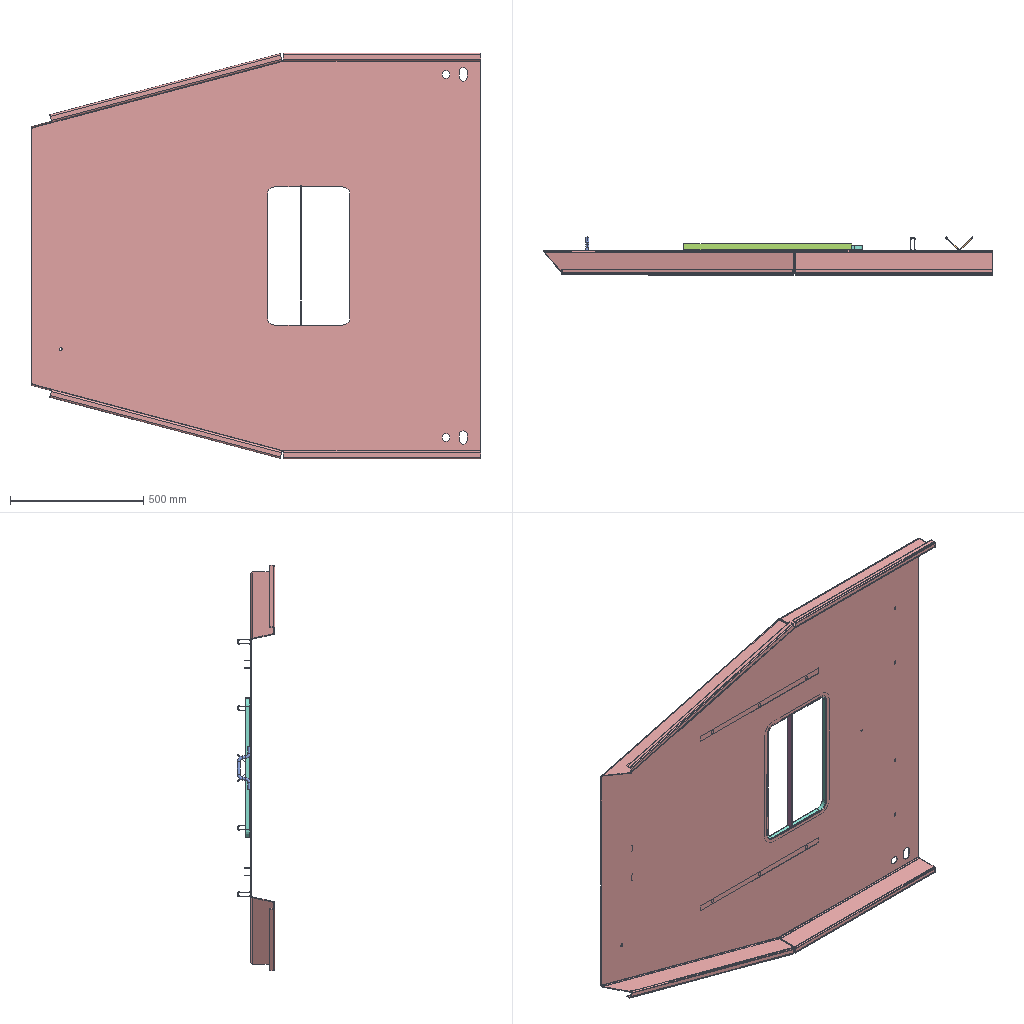Assembly | SolidWorks | 6 different items | 11 placed | box 1688 x 142 x 1525 mm
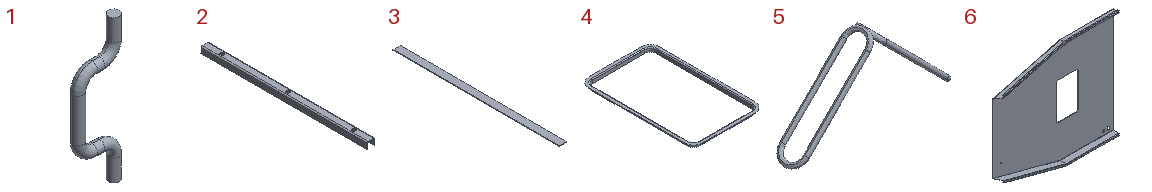Parts list (item | quantity | size | volume | features):
1 | x1 | 52 x 12 x 160 mm | 24037 mm3 | features Sweep 1
2 | x2 | 30 x 630 x 25 mm | 91837 mm3 | features EdgeFlange 1, FlatPattern 1, ICE 1, SMBaseFlange 1, SheetMetal 1
3 | x1 | 23 x 526 x 2 mm | 24196 mm3 | features FlatPattern 1, SMBaseFlange 1, SheetMetal 1
4 | x1 | 344 x 554 x 20 mm | 110720 mm3 | features Sweep 1
5 | x5 | 101.995 x 18 x 52.497 mm | 2170 mm3 | features MirrorPattern 1, RefAxis 1, Sweep 1
6 | x1 | 1688 x 90 x 1525 mm | 7493829 mm3 | features EdgeFlange 3, ICE 2, FlatPattern 1, MirrorPattern 1, SMBaseFlange 1, SheetMetal 1
Mates (type | each side: item.copy, entity, surface, feature):
Tangent | 6.1 face plane Base-Flange1 | 1.1 face cylinder Sweep1
Width | 1.1 face plane Sweep1 | 1.1 face plane Sweep1 | 6.1 face plane Edge-Flange1 | 6.1 face plane Edge-Flange1
DistanceDim | 6.1 face plane Base-Flange1 | 1.1 plane
Coincident | 6.1 face plane Base-Flange1 | 2.1 face plane Base-Flange1
DistanceDim | 2.1 face plane Edge-Flange1 | 6.1 face plane Base-Flange1
Coincident | 2.1 face plane Base-Flange1 | 2.2 face plane Base-Flange1
Coincident | 2.1 face plane Edge-Flange1 | 2.2 face plane Edge-Flange1
DistanceDim | 2.2 face plane Edge-Flange1 | 2.1 face plane Edge-Flange1
Symmetric | 6.1 plane | 2.2 face plane Edge-Flange1 | 2.1 face plane Edge-Flange1
Coincident | 4.1 face plane Sweep1 | 6.1 face plane Base-Flange1
Symmetric | 6.1 plane | 4.1 face plane Sweep1 | 4.1 face plane Sweep1
Width | 4.1 face plane Sweep1 | 4.1 face plane Sweep1 | 6.1 face plane Base-Flange1 | 6.1 face plane Base-Flange1
Coincident | 3.1 face plane Base-Flange1 | 4.1 face plane Sweep1 | 2 times
DistanceDim | 3.1 face plane Base-Flange1 | 4.1 face plane Sweep1
Coincident | 6.1 face plane Base-Flange1 | 5.1 plane
DistanceDim | 5.1 plane | 6.1 face plane Base-Flange1
DistanceDim | 5.1 plane | 6.1 plane
Coincident | 6.1 face plane Base-Flange1 | 5.2 plane
DistanceDim | 5.2 plane | 6.1 face plane Base-Flange1
Coincident | 6.1 plane | 5.2 plane